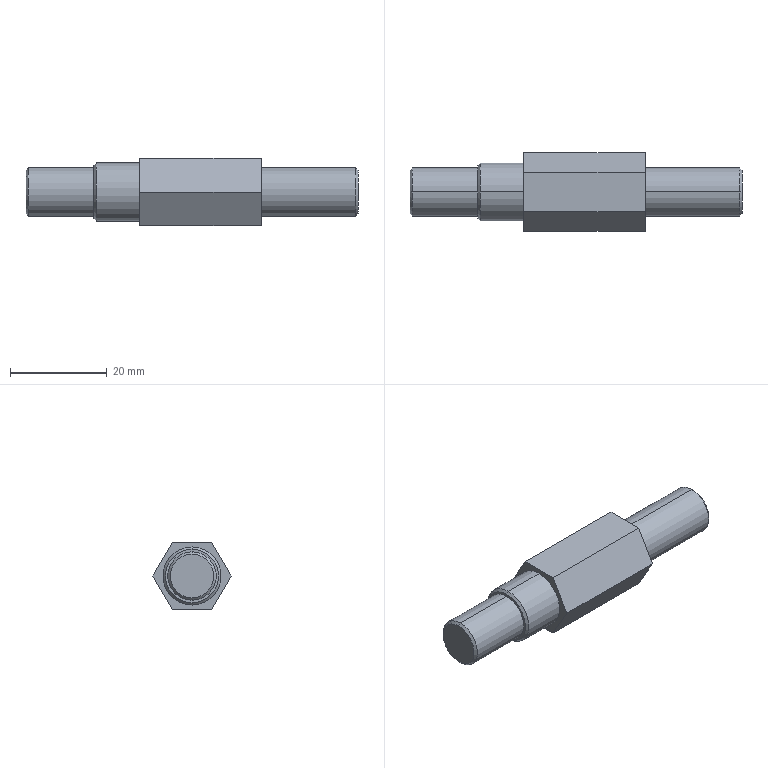Part | SolidWorks | features BaseBody 1 | 1 solid | 23 faces | box 68.5 x 16.166 x 14 mm | volume 7976 mm3 | plane 11 | cone 6 | cylinder 6 | commonest cylinder face diameters 10 x4 12 x2
STEP:
#1=CARTESIAN_POINT('',(-9.5,0.,5.5));
#2=VERTEX_POINT('',#1);
#3=CARTESIAN_POINT('',(-9.5,0.,-5.5));
#4=VERTEX_POINT('',#3);
#5=CARTESIAN_POINT('',(-9.5,0.,0.));
#6=DIRECTION('',(-1.,0.,0.));
#7=DIRECTION('',(0.,0.,1.));
#8=AXIS2_PLACEMENT_3D('',#5,#6,#7);
#9=CIRCLE('',#8,5.5);
#10=EDGE_CURVE('',#2,#4,#9,.T.);
#11=ORIENTED_EDGE('',*,*,#10,.F.);
#12=CARTESIAN_POINT('',(-9.,0.,6.));
#13=VERTEX_POINT('',#12);
#14=CARTESIAN_POINT('',(-9.5,0.,5.5));
#15=DIRECTION('',(0.7071,0.,0.7071));
#16=VECTOR('',#15,1000.);
#17=LINE('',#14,#16);
#18=EDGE_CURVE('',#2,#13,#17,.T.);
#19=ORIENTED_EDGE('',*,*,#18,.T.);
#20=CARTESIAN_POINT('',(-9.,0.,-6.));
#21=VERTEX_POINT('',#20);
#22=CARTESIAN_POINT('',(-9.,0.,0.));
#23=DIRECTION('',(1.,0.,0.));
#24=DIRECTION('',(0.,0.,1.));
#25=AXIS2_PLACEMENT_3D('',#22,#23,#24);
#26=CIRCLE('',#25,6.);
#27=EDGE_CURVE('',#21,#13,#26,.T.);
#28=ORIENTED_EDGE('',*,*,#27,.F.);
#29=CARTESIAN_POINT('',(-9.5,0.,-5.5));
#30=DIRECTION('',(0.7071,0.,-0.7071));
#31=VECTOR('',#30,1000.);
#32=LINE('',#29,#31);
#33=EDGE_CURVE('',#4,#21,#32,.T.);
#34=ORIENTED_EDGE('',*,*,#33,.F.);
#35=EDGE_LOOP('',(#11,#19,#28,#34));
#36=FACE_OUTER_BOUND('',#35,.T.);
#37=CARTESIAN_POINT('',(-9.5,0.,0.));
#38=DIRECTION('',(1.,0.,0.));
#39=DIRECTION('',(0.,0.,-1.));
#40=AXIS2_PLACEMENT_3D('',#37,#38,#39);
#41=CONICAL_SURFACE('',#40,5.5,0.7854);
#42=ADVANCED_FACE('',(#36),#41,.T.);
#43=CARTESIAN_POINT('',(-23.5,0.,4.5));
#44=VERTEX_POINT('',#43);
#45=CARTESIAN_POINT('',(-23.5,0.,-4.5));
#46=VERTEX_POINT('',#45);
#47=CARTESIAN_POINT('',(-23.5,0.,0.));
#48=DIRECTION('',(-1.,0.,0.));
#49=DIRECTION('',(0.,0.,1.));
#50=AXIS2_PLACEMENT_3D('',#47,#48,#49);
#51=CIRCLE('',#50,4.5);
#52=EDGE_CURVE('',#44,#46,#51,.T.);
#53=ORIENTED_EDGE('',*,*,#52,.F.);
#54=CARTESIAN_POINT('',(-23.,0.,5.));
#55=VERTEX_POINT('',#54);
#56=CARTESIAN_POINT('',(-23.5,0.,4.5));
#57=DIRECTION('',(0.7071,0.,0.7071));
#58=VECTOR('',#57,1000.);
#59=LINE('',#56,#58);
#60=EDGE_CURVE('',#44,#55,#59,.T.);
#61=ORIENTED_EDGE('',*,*,#60,.T.);
#62=CARTESIAN_POINT('',(-23.,0.,-5.));
#63=VERTEX_POINT('',#62);
#64=CARTESIAN_POINT('',(-23.,0.,0.));
#65=DIRECTION('',(1.,0.,0.));
#66=DIRECTION('',(0.,0.,1.));
#67=AXIS2_PLACEMENT_3D('',#64,#65,#66);
#68=CIRCLE('',#67,5.);
#69=EDGE_CURVE('',#63,#55,#68,.T.);
#70=ORIENTED_EDGE('',*,*,#69,.F.);
#71=CARTESIAN_POINT('',(-23.5,0.,-4.5));
#72=DIRECTION('',(0.7071,0.,-0.7071));
#73=VECTOR('',#72,1000.);
#74=LINE('',#71,#73);
#75=EDGE_CURVE('',#46,#63,#74,.T.);
#76=ORIENTED_EDGE('',*,*,#75,.F.);
#77=EDGE_LOOP('',(#53,#61,#70,#76));
#78=FACE_OUTER_BOUND('',#77,.T.);
#79=CARTESIAN_POINT('',(-23.5,0.,0.));
#80=DIRECTION('',(1.,0.,0.));
#81=DIRECTION('',(0.,0.,-1.));
#82=AXIS2_PLACEMENT_3D('',#79,#80,#81);
#83=CONICAL_SURFACE('',#82,4.5,0.7854);
#84=ADVANCED_FACE('',(#78),#83,.T.);
#85=CARTESIAN_POINT('',(45.,0.,-4.5));
#86=VERTEX_POINT('',#85);
#87=CARTESIAN_POINT('',(45.,0.,4.5));
#88=VERTEX_POINT('',#87);
#89=CARTESIAN_POINT('',(45.,0.,0.));
#90=DIRECTION('',(1.,0.,0.));
#91=DIRECTION('',(0.,0.,-1.));
#92=AXIS2_PLACEMENT_3D('',#89,#90,#91);
#93=CIRCLE('',#92,4.5);
#94=EDGE_CURVE('',#86,#88,#93,.T.);
#95=ORIENTED_EDGE('',*,*,#94,.F.);
#96=CARTESIAN_POINT('',(44.5,0.,-5.));
#97=VERTEX_POINT('',#96);
#98=CARTESIAN_POINT('',(45.,0.,-4.5));
#99=DIRECTION('',(-0.7071,0.,-0.7071));
#100=VECTOR('',#99,1000.);
#101=LINE('',#98,#100);
#102=EDGE_CURVE('',#86,#97,#101,.T.);
#103=ORIENTED_EDGE('',*,*,#102,.T.);
#104=CARTESIAN_POINT('',(44.5,0.,5.));
#105=VERTEX_POINT('',#104);
#106=CARTESIAN_POINT('',(44.5,0.,0.));
#107=DIRECTION('',(-1.,0.,0.));
#108=DIRECTION('',(0.,0.,-1.));
#109=AXIS2_PLACEMENT_3D('',#106,#107,#108);
#110=CIRCLE('',#109,5.);
#111=EDGE_CURVE('',#105,#97,#110,.T.);
#112=ORIENTED_EDGE('',*,*,#111,.F.);
#113=CARTESIAN_POINT('',(45.,0.,4.5));
#114=DIRECTION('',(-0.7071,0.,0.7071));
#115=VECTOR('',#114,1000.);
#116=LINE('',#113,#115);
#117=EDGE_CURVE('',#88,#105,#116,.T.);
#118=ORIENTED_EDGE('',*,*,#117,.F.);
#119=EDGE_LOOP('',(#95,#103,#112,#118));
#120=FACE_OUTER_BOUND('',#119,.T.);
#121=CARTESIAN_POINT('',(45.,0.,0.));
#122=DIRECTION('',(-1.,0.,0.));
#123=DIRECTION('',(0.,0.,1.));
#124=AXIS2_PLACEMENT_3D('',#121,#122,#123);
#125=CONICAL_SURFACE('',#124,4.5,0.7854);
#126=ADVANCED_FACE('',(#120),#125,.T.);
#127=ORIENTED_EDGE('',*,*,#111,.T.);
#128=CARTESIAN_POINT('',(25.,0.,-5.));
#129=VERTEX_POINT('',#128);
#130=CARTESIAN_POINT('',(45.,0.,-5.));
#131=DIRECTION('',(-1.,0.,0.));
#132=VECTOR('',#131,1000.);
#133=LINE('',#130,#132);
#134=EDGE_CURVE('',#97,#129,#133,.T.);
#135=ORIENTED_EDGE('',*,*,#134,.T.);
#136=CARTESIAN_POINT('',(25.,0.,5.));
#137=VERTEX_POINT('',#136);
#138=CARTESIAN_POINT('',(25.,0.,0.));
#139=DIRECTION('',(1.,0.,0.));
#140=DIRECTION('',(0.,0.,-1.));
#141=AXIS2_PLACEMENT_3D('',#138,#139,#140);
#142=CIRCLE('',#141,5.);
#143=EDGE_CURVE('',#129,#137,#142,.T.);
#144=ORIENTED_EDGE('',*,*,#143,.T.);
#145=CARTESIAN_POINT('',(45.,0.,5.));
#146=DIRECTION('',(-1.,0.,0.));
#147=VECTOR('',#146,1000.);
#148=LINE('',#145,#147);
#149=EDGE_CURVE('',#105,#137,#148,.T.);
#150=ORIENTED_EDGE('',*,*,#149,.F.);
#151=EDGE_LOOP('',(#127,#135,#144,#150));
#152=FACE_OUTER_BOUND('',#151,.T.);
#153=CARTESIAN_POINT('',(45.,0.,0.));
#154=DIRECTION('',(-1.,0.,0.));
#155=DIRECTION('',(0.,0.,1.));
#156=AXIS2_PLACEMENT_3D('',#153,#154,#155);
#157=CYLINDRICAL_SURFACE('',#156,5.);
#158=ADVANCED_FACE('',(#152),#157,.T.);
#159=ORIENTED_EDGE('',*,*,#69,.T.);
#160=CARTESIAN_POINT('',(-9.5,0.,5.));
#161=VERTEX_POINT('',#160);
#162=CARTESIAN_POINT('',(-23.5,0.,5.));
#163=DIRECTION('',(1.,0.,0.));
#164=VECTOR('',#163,1000.);
#165=LINE('',#162,#164);
#166=EDGE_CURVE('',#55,#161,#165,.T.);
#167=ORIENTED_EDGE('',*,*,#166,.T.);
#168=CARTESIAN_POINT('',(-9.5,0.,-5.));
#169=VERTEX_POINT('',#168);
#170=CARTESIAN_POINT('',(-9.5,0.,0.));
#171=DIRECTION('',(-1.,0.,0.));
#172=DIRECTION('',(0.,0.,1.));
#173=AXIS2_PLACEMENT_3D('',#170,#171,#172);
#174=CIRCLE('',#173,5.);
#175=EDGE_CURVE('',#161,#169,#174,.T.);
#176=ORIENTED_EDGE('',*,*,#175,.T.);
#177=CARTESIAN_POINT('',(-23.5,0.,-5.));
#178=DIRECTION('',(1.,0.,0.));
#179=VECTOR('',#178,1000.);
#180=LINE('',#177,#179);
#181=EDGE_CURVE('',#63,#169,#180,.T.);
#182=ORIENTED_EDGE('',*,*,#181,.F.);
#183=EDGE_LOOP('',(#159,#167,#176,#182));
#184=FACE_OUTER_BOUND('',#183,.T.);
#185=CARTESIAN_POINT('',(-23.5,0.,0.));
#186=DIRECTION('',(1.,0.,0.));
#187=DIRECTION('',(0.,0.,-1.));
#188=AXIS2_PLACEMENT_3D('',#185,#186,#187);
#189=CYLINDRICAL_SURFACE('',#188,5.);
#190=ADVANCED_FACE('',(#184),#189,.T.);
#191=ORIENTED_EDGE('',*,*,#27,.T.);
#192=CARTESIAN_POINT('',(0.,0.,6.));
#193=VERTEX_POINT('',#192);
#194=CARTESIAN_POINT('',(-9.5,0.,6.));
#195=DIRECTION('',(1.,0.,0.));
#196=VECTOR('',#195,1000.);
#197=LINE('',#194,#196);
#198=EDGE_CURVE('',#13,#193,#197,.T.);
#199=ORIENTED_EDGE('',*,*,#198,.T.);
#200=CARTESIAN_POINT('',(0.,0.,-6.));
#201=VERTEX_POINT('',#200);
#202=CARTESIAN_POINT('',(0.,0.,0.));
#203=DIRECTION('',(-1.,0.,0.));
#204=DIRECTION('',(0.,0.,-1.));
#205=AXIS2_PLACEMENT_3D('',#202,#203,#204);
#206=CIRCLE('',#205,6.);
#207=EDGE_CURVE('',#193,#201,#206,.T.);
#208=ORIENTED_EDGE('',*,*,#207,.T.);
#209=CARTESIAN_POINT('',(-9.5,0.,-6.));
#210=DIRECTION('',(1.,0.,0.));
#211=VECTOR('',#210,1000.);
#212=LINE('',#209,#211);
#213=EDGE_CURVE('',#21,#201,#212,.T.);
#214=ORIENTED_EDGE('',*,*,#213,.F.);
#215=EDGE_LOOP('',(#191,#199,#208,#214));
#216=FACE_OUTER_BOUND('',#215,.T.);
#217=CARTESIAN_POINT('',(-9.5,0.,0.));
#218=DIRECTION('',(1.,0.,0.));
#219=DIRECTION('',(0.,0.,-1.));
#220=AXIS2_PLACEMENT_3D('',#217,#218,#219);
#221=CYLINDRICAL_SURFACE('',#220,6.);
#222=ADVANCED_FACE('',(#216),#221,.T.);
#223=CARTESIAN_POINT('',(25.,4.041,-7.));
#224=VERTEX_POINT('',#223);
#225=CARTESIAN_POINT('',(25.,8.083,0.));
#226=VERTEX_POINT('',#225);
#227=CARTESIAN_POINT('',(25.,4.041,-7.));
#228=DIRECTION('',(0.,0.5,0.866));
#229=VECTOR('',#228,1000.);
#230=LINE('',#227,#229);
#231=EDGE_CURVE('',#224,#226,#230,.T.);
#232=ORIENTED_EDGE('',*,*,#231,.T.);
#233=CARTESIAN_POINT('',(25.,4.041,7.));
#234=VERTEX_POINT('',#233);
#235=CARTESIAN_POINT('',(25.,8.083,0.));
#236=DIRECTION('',(0.,-0.5,0.866));
#237=VECTOR('',#236,1000.);
#238=LINE('',#235,#237);
#239=EDGE_CURVE('',#226,#234,#238,.T.);
#240=ORIENTED_EDGE('',*,*,#239,.T.);
#241=CARTESIAN_POINT('',(25.,-4.041,7.));
#242=VERTEX_POINT('',#241);
#243=CARTESIAN_POINT('',(25.,4.041,7.));
#244=DIRECTION('',(0.,-1.,0.));
#245=VECTOR('',#244,1000.);
#246=LINE('',#243,#245);
#247=EDGE_CURVE('',#234,#242,#246,.T.);
#248=ORIENTED_EDGE('',*,*,#247,.T.);
#249=CARTESIAN_POINT('',(25.,-8.083,0.));
#250=VERTEX_POINT('',#249);
#251=CARTESIAN_POINT('',(25.,-4.041,7.));
#252=DIRECTION('',(0.,-0.5,-0.866));
#253=VECTOR('',#252,1000.);
#254=LINE('',#251,#253);
#255=EDGE_CURVE('',#242,#250,#254,.T.);
#256=ORIENTED_EDGE('',*,*,#255,.T.);
#257=CARTESIAN_POINT('',(25.,-4.041,-7.));
#258=VERTEX_POINT('',#257);
#259=CARTESIAN_POINT('',(25.,-8.083,0.));
#260=DIRECTION('',(0.,0.5,-0.866));
#261=VECTOR('',#260,1000.);
#262=LINE('',#259,#261);
#263=EDGE_CURVE('',#250,#258,#262,.T.);
#264=ORIENTED_EDGE('',*,*,#263,.T.);
#265=CARTESIAN_POINT('',(25.,-4.041,-7.));
#266=DIRECTION('',(0.,1.,0.));
#267=VECTOR('',#266,1000.);
#268=LINE('',#265,#267);
#269=EDGE_CURVE('',#258,#224,#268,.T.);
#270=ORIENTED_EDGE('',*,*,#269,.T.);
#271=EDGE_LOOP('',(#232,#240,#248,#256,#264,#270));
#272=FACE_OUTER_BOUND('',#271,.T.);
#273=CARTESIAN_POINT('',(25.,0.,0.));
#274=DIRECTION('',(1.,0.,0.));
#275=DIRECTION('',(0.,0.,-1.));
#276=AXIS2_PLACEMENT_3D('',#273,#274,#275);
#277=CIRCLE('',#276,5.);
#278=EDGE_CURVE('',#137,#129,#277,.T.);
#279=ORIENTED_EDGE('',*,*,#278,.F.);
#280=ORIENTED_EDGE('',*,*,#143,.F.);
#281=EDGE_LOOP('',(#279,#280));
#282=FACE_BOUND('',#281,.T.);
#283=CARTESIAN_POINT('',(25.,0.,0.));
#284=DIRECTION('',(1.,0.,0.));
#285=DIRECTION('',(0.,0.,-1.));
#286=AXIS2_PLACEMENT_3D('',#283,#284,#285);
#287=PLANE('',#286);
#288=ADVANCED_FACE('',(#272,#282),#287,.T.);
#289=CARTESIAN_POINT('',(-9.5,0.,0.));
#290=DIRECTION('',(-1.,0.,0.));
#291=DIRECTION('',(0.,0.,1.));
#292=AXIS2_PLACEMENT_3D('',#289,#290,#291);
#293=CIRCLE('',#292,5.5);
#294=EDGE_CURVE('',#4,#2,#293,.T.);
#295=ORIENTED_EDGE('',*,*,#294,.T.);
#296=ORIENTED_EDGE('',*,*,#10,.T.);
#297=EDGE_LOOP('',(#295,#296));
#298=FACE_OUTER_BOUND('',#297,.T.);
#299=CARTESIAN_POINT('',(-9.5,0.,0.));
#300=DIRECTION('',(-1.,0.,0.));
#301=DIRECTION('',(0.,0.,1.));
#302=AXIS2_PLACEMENT_3D('',#299,#300,#301);
#303=CIRCLE('',#302,5.);
#304=EDGE_CURVE('',#169,#161,#303,.T.);
#305=ORIENTED_EDGE('',*,*,#304,.F.);
#306=ORIENTED_EDGE('',*,*,#175,.F.);
#307=EDGE_LOOP('',(#305,#306));
#308=FACE_BOUND('',#307,.T.);
#309=CARTESIAN_POINT('',(-9.5,0.,0.));
#310=DIRECTION('',(-1.,0.,0.));
#311=DIRECTION('',(0.,0.,1.));
#312=AXIS2_PLACEMENT_3D('',#309,#310,#311);
#313=PLANE('',#312);
#314=ADVANCED_FACE('',(#298,#308),#313,.T.);
#315=CARTESIAN_POINT('',(0.,4.041,-7.));
#316=VERTEX_POINT('',#315);
#317=CARTESIAN_POINT('',(0.,8.083,0.));
#318=VERTEX_POINT('',#317);
#319=CARTESIAN_POINT('',(0.,4.041,-7.));
#320=DIRECTION('',(0.,0.5,0.866));
#321=VECTOR('',#320,1000.);
#322=LINE('',#319,#321);
#323=EDGE_CURVE('',#316,#318,#322,.T.);
#324=ORIENTED_EDGE('',*,*,#323,.F.);
#325=CARTESIAN_POINT('',(0.,-4.041,-7.));
#326=VERTEX_POINT('',#325);
#327=CARTESIAN_POINT('',(0.,-4.041,-7.));
#328=DIRECTION('',(0.,1.,0.));
#329=VECTOR('',#328,1000.);
#330=LINE('',#327,#329);
#331=EDGE_CURVE('',#326,#316,#330,.T.);
#332=ORIENTED_EDGE('',*,*,#331,.F.);
#333=CARTESIAN_POINT('',(0.,-8.083,0.));
#334=VERTEX_POINT('',#333);
#335=CARTESIAN_POINT('',(0.,-8.083,0.));
#336=DIRECTION('',(0.,0.5,-0.866));
#337=VECTOR('',#336,1000.);
#338=LINE('',#335,#337);
#339=EDGE_CURVE('',#334,#326,#338,.T.);
#340=ORIENTED_EDGE('',*,*,#339,.F.);
#341=CARTESIAN_POINT('',(0.,-4.041,7.));
#342=VERTEX_POINT('',#341);
#343=CARTESIAN_POINT('',(0.,-4.041,7.));
#344=DIRECTION('',(0.,-0.5,-0.866));
#345=VECTOR('',#344,1000.);
#346=LINE('',#343,#345);
#347=EDGE_CURVE('',#342,#334,#346,.T.);
#348=ORIENTED_EDGE('',*,*,#347,.F.);
#349=CARTESIAN_POINT('',(0.,4.041,7.));
#350=VERTEX_POINT('',#349);
#351=CARTESIAN_POINT('',(0.,4.041,7.));
#352=DIRECTION('',(0.,-1.,0.));
#353=VECTOR('',#352,1000.);
#354=LINE('',#351,#353);
#355=EDGE_CURVE('',#350,#342,#354,.T.);
#356=ORIENTED_EDGE('',*,*,#355,.F.);
#357=CARTESIAN_POINT('',(0.,8.083,0.));
#358=DIRECTION('',(0.,-0.5,0.866));
#359=VECTOR('',#358,1000.);
#360=LINE('',#357,#359);
#361=EDGE_CURVE('',#318,#350,#360,.T.);
#362=ORIENTED_EDGE('',*,*,#361,.F.);
#363=EDGE_LOOP('',(#324,#332,#340,#348,#356,#362));
#364=FACE_OUTER_BOUND('',#363,.T.);
#365=CARTESIAN_POINT('',(0.,0.,0.));
#366=DIRECTION('',(-1.,0.,0.));
#367=DIRECTION('',(0.,0.,-1.));
#368=AXIS2_PLACEMENT_3D('',#365,#366,#367);
#369=CIRCLE('',#368,6.);
#370=EDGE_CURVE('',#201,#193,#369,.T.);
#371=ORIENTED_EDGE('',*,*,#370,.F.);
#372=ORIENTED_EDGE('',*,*,#207,.F.);
#373=EDGE_LOOP('',(#371,#372));
#374=FACE_BOUND('',#373,.T.);
#375=CARTESIAN_POINT('',(0.,0.,0.));
#376=DIRECTION('',(1.,0.,0.));
#377=DIRECTION('',(0.,0.,-1.));
#378=AXIS2_PLACEMENT_3D('',#375,#376,#377);
#379=PLANE('',#378);
#380=ADVANCED_FACE('',(#364,#374),#379,.F.);
#381=ORIENTED_EDGE('',*,*,#323,.T.);
#382=CARTESIAN_POINT('',(25.,8.083,0.));
#383=DIRECTION('',(-1.,0.,0.));
#384=VECTOR('',#383,1000.);
#385=LINE('',#382,#384);
#386=EDGE_CURVE('',#226,#318,#385,.T.);
#387=ORIENTED_EDGE('',*,*,#386,.F.);
#388=ORIENTED_EDGE('',*,*,#231,.F.);
#389=CARTESIAN_POINT('',(25.,4.041,-7.));
#390=DIRECTION('',(-1.,0.,0.));
#391=VECTOR('',#390,1000.);
#392=LINE('',#389,#391);
#393=EDGE_CURVE('',#224,#316,#392,.T.);
#394=ORIENTED_EDGE('',*,*,#393,.T.);
#395=EDGE_LOOP('',(#381,#387,#388,#394));
#396=FACE_OUTER_BOUND('',#395,.T.);
#397=CARTESIAN_POINT('',(25.,4.041,-7.));
#398=DIRECTION('',(0.,-0.866,0.5));
#399=DIRECTION('',(0.,-0.5,-0.866));
#400=AXIS2_PLACEMENT_3D('',#397,#398,#399);
#401=PLANE('',#400);
#402=ADVANCED_FACE('',(#396),#401,.F.);
#403=ORIENTED_EDGE('',*,*,#361,.T.);
#404=CARTESIAN_POINT('',(25.,4.041,7.));
#405=DIRECTION('',(-1.,0.,0.));
#406=VECTOR('',#405,1000.);
#407=LINE('',#404,#406);
#408=EDGE_CURVE('',#234,#350,#407,.T.);
#409=ORIENTED_EDGE('',*,*,#408,.F.);
#410=ORIENTED_EDGE('',*,*,#239,.F.);
#411=ORIENTED_EDGE('',*,*,#386,.T.);
#412=EDGE_LOOP('',(#403,#409,#410,#411));
#413=FACE_OUTER_BOUND('',#412,.T.);
#414=CARTESIAN_POINT('',(25.,8.083,0.));
#415=DIRECTION('',(0.,-0.866,-0.5));
#416=DIRECTION('',(0.,0.5,-0.866));
#417=AXIS2_PLACEMENT_3D('',#414,#415,#416);
#418=PLANE('',#417);
#419=ADVANCED_FACE('',(#413),#418,.F.);
#420=ORIENTED_EDGE('',*,*,#355,.T.);
#421=CARTESIAN_POINT('',(25.,-4.041,7.));
#422=DIRECTION('',(-1.,0.,0.));
#423=VECTOR('',#422,1000.);
#424=LINE('',#421,#423);
#425=EDGE_CURVE('',#242,#342,#424,.T.);
#426=ORIENTED_EDGE('',*,*,#425,.F.);
#427=ORIENTED_EDGE('',*,*,#247,.F.);
#428=ORIENTED_EDGE('',*,*,#408,.T.);
#429=EDGE_LOOP('',(#420,#426,#427,#428));
#430=FACE_OUTER_BOUND('',#429,.T.);
#431=CARTESIAN_POINT('',(25.,4.041,7.));
#432=DIRECTION('',(0.,0.,-1.));
#433=DIRECTION('',(0.,1.,0.));
#434=AXIS2_PLACEMENT_3D('',#431,#432,#433);
#435=PLANE('',#434);
#436=ADVANCED_FACE('',(#430),#435,.F.);
#437=ORIENTED_EDGE('',*,*,#347,.T.);
#438=CARTESIAN_POINT('',(25.,-8.083,0.));
#439=DIRECTION('',(-1.,0.,0.));
#440=VECTOR('',#439,1000.);
#441=LINE('',#438,#440);
#442=EDGE_CURVE('',#250,#334,#441,.T.);
#443=ORIENTED_EDGE('',*,*,#442,.F.);
#444=ORIENTED_EDGE('',*,*,#255,.F.);
#445=ORIENTED_EDGE('',*,*,#425,.T.);
#446=EDGE_LOOP('',(#437,#443,#444,#445));
#447=FACE_OUTER_BOUND('',#446,.T.);
#448=CARTESIAN_POINT('',(25.,-4.041,7.));
#449=DIRECTION('',(0.,0.866,-0.5));
#450=DIRECTION('',(0.,0.5,0.866));
#451=AXIS2_PLACEMENT_3D('',#448,#449,#450);
#452=PLANE('',#451);
#453=ADVANCED_FACE('',(#447),#452,.F.);
#454=ORIENTED_EDGE('',*,*,#339,.T.);
#455=CARTESIAN_POINT('',(25.,-4.041,-7.));
#456=DIRECTION('',(-1.,0.,0.));
#457=VECTOR('',#456,1000.);
#458=LINE('',#455,#457);
#459=EDGE_CURVE('',#258,#326,#458,.T.);
#460=ORIENTED_EDGE('',*,*,#459,.F.);
#461=ORIENTED_EDGE('',*,*,#263,.F.);
#462=ORIENTED_EDGE('',*,*,#442,.T.);
#463=EDGE_LOOP('',(#454,#460,#461,#462));
#464=FACE_OUTER_BOUND('',#463,.T.);
#465=CARTESIAN_POINT('',(25.,-8.083,0.));
#466=DIRECTION('',(0.,0.866,0.5));
#467=DIRECTION('',(0.,-0.5,0.866));
#468=AXIS2_PLACEMENT_3D('',#465,#466,#467);
#469=PLANE('',#468);
#470=ADVANCED_FACE('',(#464),#469,.F.);
#471=ORIENTED_EDGE('',*,*,#331,.T.);
#472=ORIENTED_EDGE('',*,*,#393,.F.);
#473=ORIENTED_EDGE('',*,*,#269,.F.);
#474=ORIENTED_EDGE('',*,*,#459,.T.);
#475=EDGE_LOOP('',(#471,#472,#473,#474));
#476=FACE_OUTER_BOUND('',#475,.T.);
#477=CARTESIAN_POINT('',(25.,-4.041,-7.));
#478=DIRECTION('',(0.,0.,1.));
#479=DIRECTION('',(0.,-1.,0.));
#480=AXIS2_PLACEMENT_3D('',#477,#478,#479);
#481=PLANE('',#480);
#482=ADVANCED_FACE('',(#476),#481,.F.);
#483=ORIENTED_EDGE('',*,*,#198,.F.);
#484=CARTESIAN_POINT('',(-9.,0.,0.));
#485=DIRECTION('',(1.,0.,0.));
#486=DIRECTION('',(0.,0.,1.));
#487=AXIS2_PLACEMENT_3D('',#484,#485,#486);
#488=CIRCLE('',#487,6.);
#489=EDGE_CURVE('',#13,#21,#488,.T.);
#490=ORIENTED_EDGE('',*,*,#489,.T.);
#491=ORIENTED_EDGE('',*,*,#213,.T.);
#492=ORIENTED_EDGE('',*,*,#370,.T.);
#493=EDGE_LOOP('',(#483,#490,#491,#492));
#494=FACE_OUTER_BOUND('',#493,.T.);
#495=CARTESIAN_POINT('',(-9.5,0.,0.));
#496=DIRECTION('',(1.,0.,0.));
#497=DIRECTION('',(0.,0.,-1.));
#498=AXIS2_PLACEMENT_3D('',#495,#496,#497);
#499=CYLINDRICAL_SURFACE('',#498,6.);
#500=ADVANCED_FACE('',(#494),#499,.T.);
#501=ORIENTED_EDGE('',*,*,#166,.F.);
#502=CARTESIAN_POINT('',(-23.,0.,0.));
#503=DIRECTION('',(1.,0.,0.));
#504=DIRECTION('',(0.,0.,1.));
#505=AXIS2_PLACEMENT_3D('',#502,#503,#504);
#506=CIRCLE('',#505,5.);
#507=EDGE_CURVE('',#55,#63,#506,.T.);
#508=ORIENTED_EDGE('',*,*,#507,.T.);
#509=ORIENTED_EDGE('',*,*,#181,.T.);
#510=ORIENTED_EDGE('',*,*,#304,.T.);
#511=EDGE_LOOP('',(#501,#508,#509,#510));
#512=FACE_OUTER_BOUND('',#511,.T.);
#513=CARTESIAN_POINT('',(-23.5,0.,0.));
#514=DIRECTION('',(1.,0.,0.));
#515=DIRECTION('',(0.,0.,-1.));
#516=AXIS2_PLACEMENT_3D('',#513,#514,#515);
#517=CYLINDRICAL_SURFACE('',#516,5.);
#518=ADVANCED_FACE('',(#512),#517,.T.);
#519=CARTESIAN_POINT('',(-23.5,0.,0.));
#520=DIRECTION('',(-1.,0.,0.));
#521=DIRECTION('',(0.,0.,1.));
#522=AXIS2_PLACEMENT_3D('',#519,#520,#521);
#523=CIRCLE('',#522,4.5);
#524=EDGE_CURVE('',#46,#44,#523,.T.);
#525=ORIENTED_EDGE('',*,*,#524,.T.);
#526=ORIENTED_EDGE('',*,*,#52,.T.);
#527=EDGE_LOOP('',(#525,#526));
#528=FACE_OUTER_BOUND('',#527,.T.);
#529=CARTESIAN_POINT('',(-23.5,0.,0.));
#530=DIRECTION('',(-1.,0.,0.));
#531=DIRECTION('',(0.,0.,1.));
#532=AXIS2_PLACEMENT_3D('',#529,#530,#531);
#533=PLANE('',#532);
#534=ADVANCED_FACE('',(#528),#533,.T.);
#535=ORIENTED_EDGE('',*,*,#134,.F.);
#536=CARTESIAN_POINT('',(44.5,0.,0.));
#537=DIRECTION('',(-1.,0.,0.));
#538=DIRECTION('',(0.,0.,-1.));
#539=AXIS2_PLACEMENT_3D('',#536,#537,#538);
#540=CIRCLE('',#539,5.);
#541=EDGE_CURVE('',#97,#105,#540,.T.);
#542=ORIENTED_EDGE('',*,*,#541,.T.);
#543=ORIENTED_EDGE('',*,*,#149,.T.);
#544=ORIENTED_EDGE('',*,*,#278,.T.);
#545=EDGE_LOOP('',(#535,#542,#543,#544));
#546=FACE_OUTER_BOUND('',#545,.T.);
#547=CARTESIAN_POINT('',(45.,0.,0.));
#548=DIRECTION('',(-1.,0.,0.));
#549=DIRECTION('',(0.,0.,1.));
#550=AXIS2_PLACEMENT_3D('',#547,#548,#549);
#551=CYLINDRICAL_SURFACE('',#550,5.);
#552=ADVANCED_FACE('',(#546),#551,.T.);
#553=CARTESIAN_POINT('',(45.,0.,0.));
#554=DIRECTION('',(1.,0.,0.));
#555=DIRECTION('',(0.,0.,-1.));
#556=AXIS2_PLACEMENT_3D('',#553,#554,#555);
#557=CIRCLE('',#556,4.5);
#558=EDGE_CURVE('',#88,#86,#557,.T.);
#559=ORIENTED_EDGE('',*,*,#558,.T.);
#560=ORIENTED_EDGE('',*,*,#94,.T.);
#561=EDGE_LOOP('',(#559,#560));
#562=FACE_OUTER_BOUND('',#561,.T.);
#563=CARTESIAN_POINT('',(45.,0.,0.));
#564=DIRECTION('',(1.,0.,0.));
#565=DIRECTION('',(0.,0.,-1.));
#566=AXIS2_PLACEMENT_3D('',#563,#564,#565);
#567=PLANE('',#566);
#568=ADVANCED_FACE('',(#562),#567,.T.);
#569=ORIENTED_EDGE('',*,*,#102,.F.);
#570=ORIENTED_EDGE('',*,*,#558,.F.);
#571=ORIENTED_EDGE('',*,*,#117,.T.);
#572=ORIENTED_EDGE('',*,*,#541,.F.);
#573=EDGE_LOOP('',(#569,#570,#571,#572));
#574=FACE_OUTER_BOUND('',#573,.T.);
#575=CARTESIAN_POINT('',(45.,0.,0.));
#576=DIRECTION('',(-1.,0.,0.));
#577=DIRECTION('',(0.,0.,1.));
#578=AXIS2_PLACEMENT_3D('',#575,#576,#577);
#579=CONICAL_SURFACE('',#578,4.5,0.7854);
#580=ADVANCED_FACE('',(#574),#579,.T.);
#581=ORIENTED_EDGE('',*,*,#60,.F.);
#582=ORIENTED_EDGE('',*,*,#524,.F.);
#583=ORIENTED_EDGE('',*,*,#75,.T.);
#584=ORIENTED_EDGE('',*,*,#507,.F.);
#585=EDGE_LOOP('',(#581,#582,#583,#584));
#586=FACE_OUTER_BOUND('',#585,.T.);
#587=CARTESIAN_POINT('',(-23.5,0.,0.));
#588=DIRECTION('',(1.,0.,0.));
#589=DIRECTION('',(0.,0.,-1.));
#590=AXIS2_PLACEMENT_3D('',#587,#588,#589);
#591=CONICAL_SURFACE('',#590,4.5,0.7854);
#592=ADVANCED_FACE('',(#586),#591,.T.);
#593=ORIENTED_EDGE('',*,*,#18,.F.);
#594=ORIENTED_EDGE('',*,*,#294,.F.);
#595=ORIENTED_EDGE('',*,*,#33,.T.);
#596=ORIENTED_EDGE('',*,*,#489,.F.);
#597=EDGE_LOOP('',(#593,#594,#595,#596));
#598=FACE_OUTER_BOUND('',#597,.T.);
#599=CARTESIAN_POINT('',(-9.5,0.,0.));
#600=DIRECTION('',(1.,0.,0.));
#601=DIRECTION('',(0.,0.,-1.));
#602=AXIS2_PLACEMENT_3D('',#599,#600,#601);
#603=CONICAL_SURFACE('',#602,5.5,0.7854);
#604=ADVANCED_FACE('',(#598),#603,.T.);
#605=CLOSED_SHELL('',(#42,#84,#126,#158,#190,#222,#288,#314,#380,#402,#419,#436,#453,#470,#482,#500,#518,#534,#552,#568,#580,#592,#604));
#606=MANIFOLD_SOLID_BREP('',#605);
#607=CARTESIAN_POINT('',(0.,0.,0.));
#608=DIRECTION('',(0.,0.,1.));
#609=DIRECTION('',(1.,0.,0.));
#610=AXIS2_PLACEMENT_3D('',#607,#608,#609);
#611=(LENGTH_UNIT()NAMED_UNIT(*)SI_UNIT(.MILLI.,.METRE.));
#612=UNCERTAINTY_MEASURE_WITH_UNIT(LENGTH_MEASURE(0.00001),#611,'','');
#613=(NAMED_UNIT(*)PLANE_ANGLE_UNIT()SI_UNIT($,.RADIAN.));
#614=(NAMED_UNIT(*)SI_UNIT($,.STERADIAN.)SOLID_ANGLE_UNIT());
#615=(GEOMETRIC_REPRESENTATION_CONTEXT(3)GLOBAL_UNCERTAINTY_ASSIGNED_CONTEXT((#612))GLOBAL_UNIT_ASSIGNED_CONTEXT((#611,#613,#614))REPRESENTATION_CONTEXT('',''));
#616=ADVANCED_BREP_SHAPE_REPRESENTATION('',(#606,#610),#615);